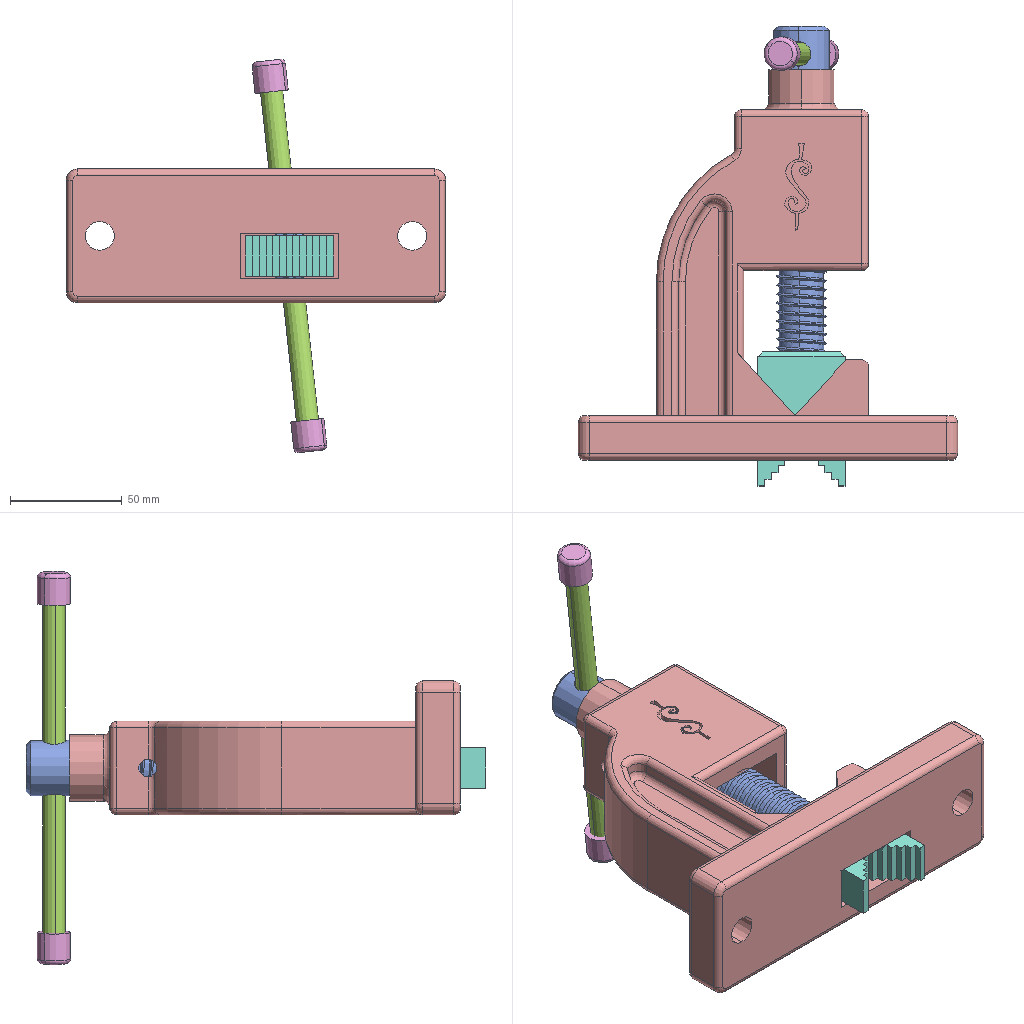Assembly | SolidWorks | 5 different items | 6 placed | box 170 x 206 x 176 mm
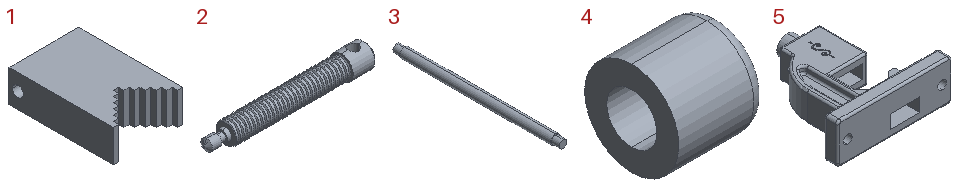Parts list (item | quantity | size | volume | features):
1 | x1 | 39 x 60 x 18 mm | 32904 mm3 | features Chamfer 1, Extrusion 1, ICE 1, RevCut 1
2 | x1 | 169.464 x 25 x 25 mm | 51868 mm3 | features Chamfer 1, Helix 1, ICE 1, Revolution 1, Sweep 1
3 | x1 | 10 x 172 x 10 mm | 13056 mm3 | features Extrusion 1, ICE 1, MirrorPattern 1
4 | x2 | 14 x 15 x 15 mm | 1834 mm3 | features Revolution 1
5 | x1 | 170 x 175 x 60 mm | 453597 mm3 | features ICE 8, Fillet 2, Extrusion 1, Helix 1, MirrorPattern 1, SweepCut 1
Mates (type | each side: item.copy, entity, surface, feature):
Concentric | 5.1 face cylinder Boss-Extrude3 | 2.1 face cylinder Revolve1
Concentric | 2.1 face cylinder Cut-Extrude1 | 3.1 face cylinder Boss-Extrude1
Coincident | 2.1 plane | 3.1 plane
Concentric | 3.1 face cylinder Boss-Extrude2 | 4.1 face cylinder Revolve1
Coincident | 3.1 face plane Boss-Extrude2 | 4.1 face plane Revolve1
Concentric | 3.1 face cylinder Mirror1 | 4.2 face cylinder Revolve1
Coincident | 3.1 face plane Mirror1 | 4.2 face plane Revolve1
Screw | 5.1 face cylinder Cut-Extrude4 | 2.1 face cylinder Revolve1
Coincident | 2.1 face cone Revolve1 | 1.1 face cone Cut-Revolve1
Parallel | 5.1 face plane Boss-Extrude2 | 1.1 face plane Boss-Extrude1